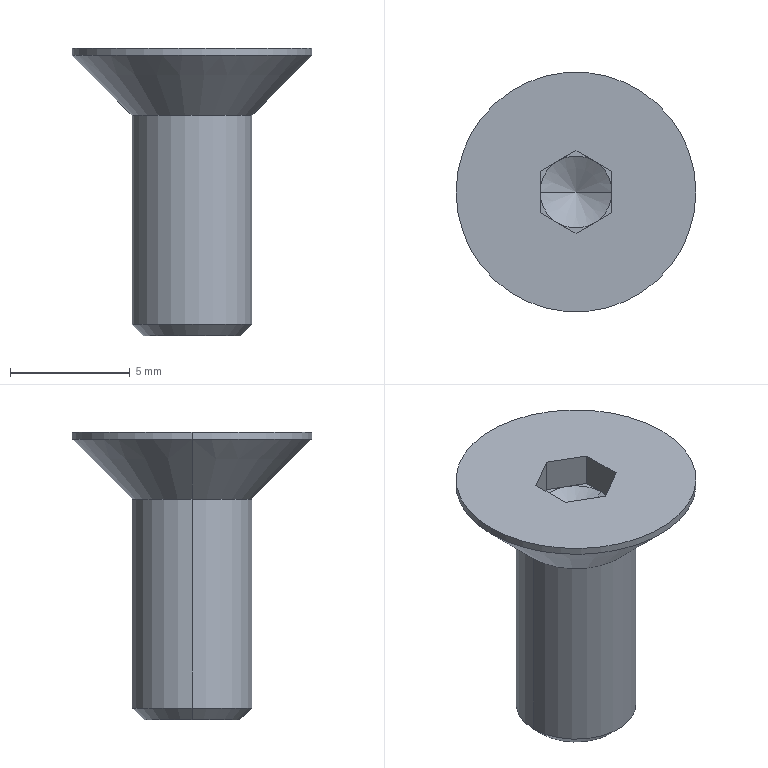Part | SolidWorks | features BaseBody 1 | 1 solid | 24 faces | box 10 x 10 x 12 mm | volume 304.022 mm3 | plane 14 | cone 6 | cylinder 4 | commonest cylinder face diameters 5 x2 10 x2
STEP:
#1=CARTESIAN_POINT('',(2.5,0.,-8.71));
#2=VERTEX_POINT('',#1);
#3=CARTESIAN_POINT('',(-2.5,0.,-8.71));
#4=VERTEX_POINT('',#3);
#5=CARTESIAN_POINT('',(0.,0.,-8.71));
#6=DIRECTION('',(0.,0.,1.));
#7=DIRECTION('',(1.,0.,0.));
#8=AXIS2_PLACEMENT_3D('',#5,#6,#7);
#9=CIRCLE('',#8,2.5);
#10=EDGE_CURVE('',#2,#4,#9,.T.);
#11=ORIENTED_EDGE('',*,*,#10,.T.);
#12=CARTESIAN_POINT('',(-2.5,0.,0.));
#13=VERTEX_POINT('',#12);
#14=CARTESIAN_POINT('',(-2.5,0.,-9.2));
#15=DIRECTION('',(0.,0.,1.));
#16=VECTOR('',#15,1000.);
#17=LINE('',#14,#16);
#18=EDGE_CURVE('',#4,#13,#17,.T.);
#19=ORIENTED_EDGE('',*,*,#18,.T.);
#20=CARTESIAN_POINT('',(2.5,0.,0.));
#21=VERTEX_POINT('',#20);
#22=CARTESIAN_POINT('',(0.,0.,0.));
#23=DIRECTION('',(0.,0.,-1.));
#24=DIRECTION('',(1.,0.,0.));
#25=AXIS2_PLACEMENT_3D('',#22,#23,#24);
#26=CIRCLE('',#25,2.5);
#27=EDGE_CURVE('',#13,#21,#26,.T.);
#28=ORIENTED_EDGE('',*,*,#27,.T.);
#29=CARTESIAN_POINT('',(2.5,0.,-9.2));
#30=DIRECTION('',(0.,0.,1.));
#31=VECTOR('',#30,1000.);
#32=LINE('',#29,#31);
#33=EDGE_CURVE('',#2,#21,#32,.T.);
#34=ORIENTED_EDGE('',*,*,#33,.F.);
#35=EDGE_LOOP('',(#11,#19,#28,#34));
#36=FACE_OUTER_BOUND('',#35,.T.);
#37=CARTESIAN_POINT('',(0.,0.,-9.2));
#38=DIRECTION('',(0.,0.,1.));
#39=DIRECTION('',(1.,0.,0.));
#40=AXIS2_PLACEMENT_3D('',#37,#38,#39);
#41=CYLINDRICAL_SURFACE('',#40,2.5);
#42=ADVANCED_FACE('',(#36),#41,.T.);
#43=ORIENTED_EDGE('',*,*,#27,.F.);
#44=CARTESIAN_POINT('',(-5.,0.,2.5));
#45=VERTEX_POINT('',#44);
#46=CARTESIAN_POINT('',(-5.,0.,2.5));
#47=DIRECTION('',(-0.7071,0.,0.7071));
#48=VECTOR('',#47,1000.);
#49=LINE('',#46,#48);
#50=EDGE_CURVE('',#13,#45,#49,.T.);
#51=ORIENTED_EDGE('',*,*,#50,.T.);
#52=CARTESIAN_POINT('',(5.,0.,2.5));
#53=VERTEX_POINT('',#52);
#54=CARTESIAN_POINT('',(0.,0.,2.5));
#55=DIRECTION('',(0.,0.,-1.));
#56=DIRECTION('',(1.,0.,0.));
#57=AXIS2_PLACEMENT_3D('',#54,#55,#56);
#58=CIRCLE('',#57,5.);
#59=EDGE_CURVE('',#45,#53,#58,.T.);
#60=ORIENTED_EDGE('',*,*,#59,.T.);
#61=CARTESIAN_POINT('',(5.,0.,2.5));
#62=DIRECTION('',(0.7071,0.,0.7071));
#63=VECTOR('',#62,1000.);
#64=LINE('',#61,#63);
#65=EDGE_CURVE('',#21,#53,#64,.T.);
#66=ORIENTED_EDGE('',*,*,#65,.F.);
#67=EDGE_LOOP('',(#43,#51,#60,#66));
#68=FACE_OUTER_BOUND('',#67,.T.);
#69=CARTESIAN_POINT('',(0.,0.,2.5));
#70=DIRECTION('',(0.,0.,1.));
#71=DIRECTION('',(1.,0.,0.));
#72=AXIS2_PLACEMENT_3D('',#69,#70,#71);
#73=CONICAL_SURFACE('',#72,5.,0.7854);
#74=ADVANCED_FACE('',(#68),#73,.T.);
#75=CARTESIAN_POINT('',(2.009,0.,-9.2));
#76=VERTEX_POINT('',#75);
#77=CARTESIAN_POINT('',(-2.009,0.,-9.2));
#78=VERTEX_POINT('',#77);
#79=CARTESIAN_POINT('',(0.,0.,-9.2));
#80=DIRECTION('',(0.,0.,1.));
#81=DIRECTION('',(1.,0.,0.));
#82=AXIS2_PLACEMENT_3D('',#79,#80,#81);
#83=CIRCLE('',#82,2.009);
#84=EDGE_CURVE('',#76,#78,#83,.T.);
#85=ORIENTED_EDGE('',*,*,#84,.T.);
#86=CARTESIAN_POINT('',(-2.5,0.,-8.71));
#87=DIRECTION('',(-0.7071,0.,0.7071));
#88=VECTOR('',#87,1000.);
#89=LINE('',#86,#88);
#90=EDGE_CURVE('',#78,#4,#89,.T.);
#91=ORIENTED_EDGE('',*,*,#90,.T.);
#92=ORIENTED_EDGE('',*,*,#10,.F.);
#93=CARTESIAN_POINT('',(2.5,0.,-8.71));
#94=DIRECTION('',(0.7071,0.,0.7071));
#95=VECTOR('',#94,1000.);
#96=LINE('',#93,#95);
#97=EDGE_CURVE('',#76,#2,#96,.T.);
#98=ORIENTED_EDGE('',*,*,#97,.F.);
#99=EDGE_LOOP('',(#85,#91,#92,#98));
#100=FACE_OUTER_BOUND('',#99,.T.);
#101=CARTESIAN_POINT('',(0.,0.,-8.71));
#102=DIRECTION('',(0.,0.,1.));
#103=DIRECTION('',(1.,0.,0.));
#104=AXIS2_PLACEMENT_3D('',#101,#102,#103);
#105=CONICAL_SURFACE('',#104,2.5,0.7854);
#106=ADVANCED_FACE('',(#100),#105,.T.);
#107=ORIENTED_EDGE('',*,*,#59,.F.);
#108=CARTESIAN_POINT('',(-5.,0.,2.8));
#109=VERTEX_POINT('',#108);
#110=CARTESIAN_POINT('',(-5.,0.,0.));
#111=DIRECTION('',(0.,0.,1.));
#112=VECTOR('',#111,1000.);
#113=LINE('',#110,#112);
#114=EDGE_CURVE('',#45,#109,#113,.T.);
#115=ORIENTED_EDGE('',*,*,#114,.T.);
#116=CARTESIAN_POINT('',(5.,0.,2.8));
#117=VERTEX_POINT('',#116);
#118=CARTESIAN_POINT('',(0.,0.,2.8));
#119=DIRECTION('',(0.,0.,-1.));
#120=DIRECTION('',(1.,0.,0.));
#121=AXIS2_PLACEMENT_3D('',#118,#119,#120);
#122=CIRCLE('',#121,5.);
#123=EDGE_CURVE('',#109,#117,#122,.T.);
#124=ORIENTED_EDGE('',*,*,#123,.T.);
#125=CARTESIAN_POINT('',(5.,0.,0.));
#126=DIRECTION('',(0.,0.,1.));
#127=VECTOR('',#126,1000.);
#128=LINE('',#125,#127);
#129=EDGE_CURVE('',#53,#117,#128,.T.);
#130=ORIENTED_EDGE('',*,*,#129,.F.);
#131=EDGE_LOOP('',(#107,#115,#124,#130));
#132=FACE_OUTER_BOUND('',#131,.T.);
#133=CARTESIAN_POINT('',(0.,0.,0.));
#134=DIRECTION('',(0.,0.,1.));
#135=DIRECTION('',(1.,0.,0.));
#136=AXIS2_PLACEMENT_3D('',#133,#134,#135);
#137=CYLINDRICAL_SURFACE('',#136,5.);
#138=ADVANCED_FACE('',(#132),#137,.T.);
#139=CARTESIAN_POINT('',(0.,0.,0.534));
#140=VERTEX_POINT('',#139);
#141=CARTESIAN_POINT('',(1.5,0.,1.4));
#142=VERTEX_POINT('',#141);
#143=CARTESIAN_POINT('',(1.5,0.,1.4));
#144=DIRECTION('',(0.866,0.,0.5));
#145=VECTOR('',#144,1000.);
#146=LINE('',#143,#145);
#147=EDGE_CURVE('',#140,#142,#146,.T.);
#148=ORIENTED_EDGE('',*,*,#147,.F.);
#149=CARTESIAN_POINT('',(-1.5,0.,1.4));
#150=VERTEX_POINT('',#149);
#151=CARTESIAN_POINT('',(-1.5,0.,1.4));
#152=DIRECTION('',(-0.866,0.,0.5));
#153=VECTOR('',#152,1000.);
#154=LINE('',#151,#153);
#155=EDGE_CURVE('',#140,#150,#154,.T.);
#156=ORIENTED_EDGE('',*,*,#155,.T.);
#157=CARTESIAN_POINT('',(-0.75,-1.299,1.4));
#158=VERTEX_POINT('',#157);
#159=CARTESIAN_POINT('',(0.,0.,1.4));
#160=DIRECTION('',(0.,0.,-1.));
#161=DIRECTION('',(1.,0.,0.));
#162=AXIS2_PLACEMENT_3D('',#159,#160,#161);
#163=CIRCLE('',#162,1.5);
#164=EDGE_CURVE('',#158,#150,#163,.T.);
#165=ORIENTED_EDGE('',*,*,#164,.F.);
#166=CARTESIAN_POINT('',(0.75,-1.299,1.4));
#167=VERTEX_POINT('',#166);
#168=CARTESIAN_POINT('',(0.,0.,1.4));
#169=DIRECTION('',(0.,0.,-1.));
#170=DIRECTION('',(1.,0.,0.));
#171=AXIS2_PLACEMENT_3D('',#168,#169,#170);
#172=CIRCLE('',#171,1.5);
#173=EDGE_CURVE('',#167,#158,#172,.T.);
#174=ORIENTED_EDGE('',*,*,#173,.F.);
#175=CARTESIAN_POINT('',(0.,0.,1.4));
#176=DIRECTION('',(0.,0.,-1.));
#177=DIRECTION('',(1.,0.,0.));
#178=AXIS2_PLACEMENT_3D('',#175,#176,#177);
#179=CIRCLE('',#178,1.5);
#180=EDGE_CURVE('',#142,#167,#179,.T.);
#181=ORIENTED_EDGE('',*,*,#180,.F.);
#182=EDGE_LOOP('',(#148,#156,#165,#174,#181));
#183=FACE_OUTER_BOUND('',#182,.T.);
#184=CARTESIAN_POINT('',(0.,0.,1.4));
#185=DIRECTION('',(0.,0.,1.));
#186=DIRECTION('',(1.,0.,0.));
#187=AXIS2_PLACEMENT_3D('',#184,#185,#186);
#188=CONICAL_SURFACE('',#187,1.5,1.047);
#189=ADVANCED_FACE('',(#183),#188,.F.);
#190=ORIENTED_EDGE('',*,*,#18,.F.);
#191=CARTESIAN_POINT('',(0.,0.,-8.71));
#192=DIRECTION('',(0.,0.,1.));
#193=DIRECTION('',(1.,0.,0.));
#194=AXIS2_PLACEMENT_3D('',#191,#192,#193);
#195=CIRCLE('',#194,2.5);
#196=EDGE_CURVE('',#4,#2,#195,.T.);
#197=ORIENTED_EDGE('',*,*,#196,.T.);
#198=ORIENTED_EDGE('',*,*,#33,.T.);
#199=CARTESIAN_POINT('',(0.,0.,0.));
#200=DIRECTION('',(0.,0.,-1.));
#201=DIRECTION('',(1.,0.,0.));
#202=AXIS2_PLACEMENT_3D('',#199,#200,#201);
#203=CIRCLE('',#202,2.5);
#204=EDGE_CURVE('',#21,#13,#203,.T.);
#205=ORIENTED_EDGE('',*,*,#204,.T.);
#206=EDGE_LOOP('',(#190,#197,#198,#205));
#207=FACE_OUTER_BOUND('',#206,.T.);
#208=CARTESIAN_POINT('',(0.,0.,-9.2));
#209=DIRECTION('',(0.,0.,1.));
#210=DIRECTION('',(1.,0.,0.));
#211=AXIS2_PLACEMENT_3D('',#208,#209,#210);
#212=CYLINDRICAL_SURFACE('',#211,2.5);
#213=ADVANCED_FACE('',(#207),#212,.T.);
#214=ORIENTED_EDGE('',*,*,#50,.F.);
#215=ORIENTED_EDGE('',*,*,#204,.F.);
#216=ORIENTED_EDGE('',*,*,#65,.T.);
#217=CARTESIAN_POINT('',(0.,0.,2.5));
#218=DIRECTION('',(0.,0.,-1.));
#219=DIRECTION('',(1.,0.,0.));
#220=AXIS2_PLACEMENT_3D('',#217,#218,#219);
#221=CIRCLE('',#220,5.);
#222=EDGE_CURVE('',#53,#45,#221,.T.);
#223=ORIENTED_EDGE('',*,*,#222,.T.);
#224=EDGE_LOOP('',(#214,#215,#216,#223));
#225=FACE_OUTER_BOUND('',#224,.T.);
#226=CARTESIAN_POINT('',(0.,0.,2.5));
#227=DIRECTION('',(0.,0.,1.));
#228=DIRECTION('',(1.,0.,0.));
#229=AXIS2_PLACEMENT_3D('',#226,#227,#228);
#230=CONICAL_SURFACE('',#229,5.,0.7854);
#231=ADVANCED_FACE('',(#225),#230,.T.);
#232=ORIENTED_EDGE('',*,*,#90,.F.);
#233=CARTESIAN_POINT('',(0.,0.,-9.2));
#234=DIRECTION('',(0.,0.,1.));
#235=DIRECTION('',(1.,0.,0.));
#236=AXIS2_PLACEMENT_3D('',#233,#234,#235);
#237=CIRCLE('',#236,2.009);
#238=EDGE_CURVE('',#78,#76,#237,.T.);
#239=ORIENTED_EDGE('',*,*,#238,.T.);
#240=ORIENTED_EDGE('',*,*,#97,.T.);
#241=ORIENTED_EDGE('',*,*,#196,.F.);
#242=EDGE_LOOP('',(#232,#239,#240,#241));
#243=FACE_OUTER_BOUND('',#242,.T.);
#244=CARTESIAN_POINT('',(0.,0.,-8.71));
#245=DIRECTION('',(0.,0.,1.));
#246=DIRECTION('',(1.,0.,0.));
#247=AXIS2_PLACEMENT_3D('',#244,#245,#246);
#248=CONICAL_SURFACE('',#247,2.5,0.7854);
#249=ADVANCED_FACE('',(#243),#248,.T.);
#250=ORIENTED_EDGE('',*,*,#114,.F.);
#251=ORIENTED_EDGE('',*,*,#222,.F.);
#252=ORIENTED_EDGE('',*,*,#129,.T.);
#253=CARTESIAN_POINT('',(0.,0.,2.8));
#254=DIRECTION('',(0.,0.,-1.));
#255=DIRECTION('',(1.,0.,0.));
#256=AXIS2_PLACEMENT_3D('',#253,#254,#255);
#257=CIRCLE('',#256,5.);
#258=EDGE_CURVE('',#117,#109,#257,.T.);
#259=ORIENTED_EDGE('',*,*,#258,.T.);
#260=EDGE_LOOP('',(#250,#251,#252,#259));
#261=FACE_OUTER_BOUND('',#260,.T.);
#262=CARTESIAN_POINT('',(0.,0.,0.));
#263=DIRECTION('',(0.,0.,1.));
#264=DIRECTION('',(1.,0.,0.));
#265=AXIS2_PLACEMENT_3D('',#262,#263,#264);
#266=CYLINDRICAL_SURFACE('',#265,5.);
#267=ADVANCED_FACE('',(#261),#266,.T.);
#268=ORIENTED_EDGE('',*,*,#84,.F.);
#269=ORIENTED_EDGE('',*,*,#238,.F.);
#270=EDGE_LOOP('',(#268,#269));
#271=FACE_OUTER_BOUND('',#270,.T.);
#272=CARTESIAN_POINT('',(0.,2.01,-9.2));
#273=DIRECTION('',(0.,0.,1.));
#274=DIRECTION('',(1.,0.,0.));
#275=AXIS2_PLACEMENT_3D('',#272,#273,#274);
#276=PLANE('',#275);
#277=ADVANCED_FACE('',(#271),#276,.F.);
#278=CARTESIAN_POINT('',(-1.5,-0.866,2.8));
#279=VERTEX_POINT('',#278);
#280=CARTESIAN_POINT('',(0.,-1.732,2.8));
#281=VERTEX_POINT('',#280);
#282=CARTESIAN_POINT('',(-1.5,-0.866,2.8));
#283=DIRECTION('',(0.866,-0.5,0.));
#284=VECTOR('',#283,1000.);
#285=LINE('',#282,#284);
#286=EDGE_CURVE('',#279,#281,#285,.T.);
#287=ORIENTED_EDGE('',*,*,#286,.F.);
#288=CARTESIAN_POINT('',(-1.5,0.866,2.8));
#289=VERTEX_POINT('',#288);
#290=CARTESIAN_POINT('',(-1.5,0.,2.8));
#291=DIRECTION('',(0.,-1.,0.));
#292=VECTOR('',#291,1000.);
#293=LINE('',#290,#292);
#294=EDGE_CURVE('',#289,#279,#293,.T.);
#295=ORIENTED_EDGE('',*,*,#294,.F.);
#296=CARTESIAN_POINT('',(0.,1.732,2.8));
#297=VERTEX_POINT('',#296);
#298=CARTESIAN_POINT('',(0.,1.732,2.8));
#299=DIRECTION('',(-0.866,-0.5,0.));
#300=VECTOR('',#299,1000.);
#301=LINE('',#298,#300);
#302=EDGE_CURVE('',#297,#289,#301,.T.);
#303=ORIENTED_EDGE('',*,*,#302,.F.);
#304=CARTESIAN_POINT('',(1.5,0.866,2.8));
#305=VERTEX_POINT('',#304);
#306=CARTESIAN_POINT('',(1.5,0.866,2.8));
#307=DIRECTION('',(-0.866,0.5,0.));
#308=VECTOR('',#307,1000.);
#309=LINE('',#306,#308);
#310=EDGE_CURVE('',#305,#297,#309,.T.);
#311=ORIENTED_EDGE('',*,*,#310,.F.);
#312=CARTESIAN_POINT('',(1.5,-0.866,2.8));
#313=VERTEX_POINT('',#312);
#314=CARTESIAN_POINT('',(1.5,0.,2.8));
#315=DIRECTION('',(0.,1.,0.));
#316=VECTOR('',#315,1000.);
#317=LINE('',#314,#316);
#318=EDGE_CURVE('',#313,#305,#317,.T.);
#319=ORIENTED_EDGE('',*,*,#318,.F.);
#320=CARTESIAN_POINT('',(0.,-1.732,2.8));
#321=DIRECTION('',(0.866,0.5,0.));
#322=VECTOR('',#321,1000.);
#323=LINE('',#320,#322);
#324=EDGE_CURVE('',#281,#313,#323,.T.);
#325=ORIENTED_EDGE('',*,*,#324,.F.);
#326=EDGE_LOOP('',(#287,#295,#303,#311,#319,#325));
#327=FACE_BOUND('',#326,.T.);
#328=ORIENTED_EDGE('',*,*,#258,.F.);
#329=ORIENTED_EDGE('',*,*,#123,.F.);
#330=EDGE_LOOP('',(#328,#329));
#331=FACE_OUTER_BOUND('',#330,.T.);
#332=CARTESIAN_POINT('',(0.,0.,2.8));
#333=DIRECTION('',(0.,0.,-1.));
#334=DIRECTION('',(-1.,0.,0.));
#335=AXIS2_PLACEMENT_3D('',#332,#333,#334);
#336=PLANE('',#335);
#337=ADVANCED_FACE('',(#327,#331),#336,.F.);
#338=CARTESIAN_POINT('',(1.5,-0.866,1.4));
#339=VERTEX_POINT('',#338);
#340=CARTESIAN_POINT('',(1.5,-0.866,1.4));
#341=DIRECTION('',(0.,0.,1.));
#342=VECTOR('',#341,1000.);
#343=LINE('',#340,#342);
#344=EDGE_CURVE('',#339,#313,#343,.T.);
#345=ORIENTED_EDGE('',*,*,#344,.F.);
#346=CARTESIAN_POINT('',(0.,-1.732,1.4));
#347=DIRECTION('',(0.866,0.5,0.));
#348=VECTOR('',#347,1000.);
#349=LINE('',#346,#348);
#350=EDGE_CURVE('',#167,#339,#349,.T.);
#351=ORIENTED_EDGE('',*,*,#350,.F.);
#352=CARTESIAN_POINT('',(0.,-1.732,1.4));
#353=VERTEX_POINT('',#352);
#354=CARTESIAN_POINT('',(0.,-1.732,1.4));
#355=DIRECTION('',(0.866,0.5,0.));
#356=VECTOR('',#355,1000.);
#357=LINE('',#354,#356);
#358=EDGE_CURVE('',#353,#167,#357,.T.);
#359=ORIENTED_EDGE('',*,*,#358,.F.);
#360=CARTESIAN_POINT('',(0.,-1.732,1.4));
#361=DIRECTION('',(0.,0.,-1.));
#362=VECTOR('',#361,1000.);
#363=LINE('',#360,#362);
#364=EDGE_CURVE('',#281,#353,#363,.T.);
#365=ORIENTED_EDGE('',*,*,#364,.F.);
#366=ORIENTED_EDGE('',*,*,#324,.T.);
#367=EDGE_LOOP('',(#345,#351,#359,#365,#366));
#368=FACE_OUTER_BOUND('',#367,.T.);
#369=CARTESIAN_POINT('',(0.,-1.732,1.4));
#370=DIRECTION('',(0.5,-0.866,0.));
#371=DIRECTION('',(0.866,0.5,0.));
#372=AXIS2_PLACEMENT_3D('',#369,#370,#371);
#373=PLANE('',#372);
#374=ADVANCED_FACE('',(#368),#373,.F.);
#375=ORIENTED_EDGE('',*,*,#364,.T.);
#376=CARTESIAN_POINT('',(-1.5,-0.866,1.4));
#377=DIRECTION('',(0.866,-0.5,0.));
#378=VECTOR('',#377,1000.);
#379=LINE('',#376,#378);
#380=EDGE_CURVE('',#158,#353,#379,.T.);
#381=ORIENTED_EDGE('',*,*,#380,.F.);
#382=CARTESIAN_POINT('',(-1.5,-0.866,1.4));
#383=VERTEX_POINT('',#382);
#384=CARTESIAN_POINT('',(-1.5,-0.866,1.4));
#385=DIRECTION('',(0.866,-0.5,0.));
#386=VECTOR('',#385,1000.);
#387=LINE('',#384,#386);
#388=EDGE_CURVE('',#383,#158,#387,.T.);
#389=ORIENTED_EDGE('',*,*,#388,.F.);
#390=CARTESIAN_POINT('',(-1.5,-0.866,1.4));
#391=DIRECTION('',(0.,0.,-1.));
#392=VECTOR('',#391,1000.);
#393=LINE('',#390,#392);
#394=EDGE_CURVE('',#279,#383,#393,.T.);
#395=ORIENTED_EDGE('',*,*,#394,.F.);
#396=ORIENTED_EDGE('',*,*,#286,.T.);
#397=EDGE_LOOP('',(#375,#381,#389,#395,#396));
#398=FACE_OUTER_BOUND('',#397,.T.);
#399=CARTESIAN_POINT('',(-1.5,-0.866,1.4));
#400=DIRECTION('',(-0.5,-0.866,0.));
#401=DIRECTION('',(0.866,-0.5,0.));
#402=AXIS2_PLACEMENT_3D('',#399,#400,#401);
#403=PLANE('',#402);
#404=ADVANCED_FACE('',(#398),#403,.F.);
#405=ORIENTED_EDGE('',*,*,#394,.T.);
#406=CARTESIAN_POINT('',(-1.5,0.866,1.4));
#407=DIRECTION('',(0.,-1.,0.));
#408=VECTOR('',#407,1000.);
#409=LINE('',#406,#408);
#410=EDGE_CURVE('',#150,#383,#409,.T.);
#411=ORIENTED_EDGE('',*,*,#410,.F.);
#412=CARTESIAN_POINT('',(-1.5,0.866,1.4));
#413=VERTEX_POINT('',#412);
#414=CARTESIAN_POINT('',(-1.5,0.866,1.4));
#415=DIRECTION('',(0.,-1.,0.));
#416=VECTOR('',#415,1000.);
#417=LINE('',#414,#416);
#418=EDGE_CURVE('',#413,#150,#417,.T.);
#419=ORIENTED_EDGE('',*,*,#418,.F.);
#420=CARTESIAN_POINT('',(-1.5,0.866,1.4));
#421=DIRECTION('',(0.,0.,-1.));
#422=VECTOR('',#421,1000.);
#423=LINE('',#420,#422);
#424=EDGE_CURVE('',#289,#413,#423,.T.);
#425=ORIENTED_EDGE('',*,*,#424,.F.);
#426=ORIENTED_EDGE('',*,*,#294,.T.);
#427=EDGE_LOOP('',(#405,#411,#419,#425,#426));
#428=FACE_OUTER_BOUND('',#427,.T.);
#429=CARTESIAN_POINT('',(-1.5,0.866,1.4));
#430=DIRECTION('',(-1.,0.,0.));
#431=DIRECTION('',(0.,0.,1.));
#432=AXIS2_PLACEMENT_3D('',#429,#430,#431);
#433=PLANE('',#432);
#434=ADVANCED_FACE('',(#428),#433,.F.);
#435=ORIENTED_EDGE('',*,*,#424,.T.);
#436=CARTESIAN_POINT('',(-0.75,1.299,1.4));
#437=VERTEX_POINT('',#436);
#438=CARTESIAN_POINT('',(0.,1.732,1.4));
#439=DIRECTION('',(-0.866,-0.5,0.));
#440=VECTOR('',#439,1000.);
#441=LINE('',#438,#440);
#442=EDGE_CURVE('',#437,#413,#441,.T.);
#443=ORIENTED_EDGE('',*,*,#442,.F.);
#444=CARTESIAN_POINT('',(0.,1.732,1.4));
#445=VERTEX_POINT('',#444);
#446=CARTESIAN_POINT('',(0.,1.732,1.4));
#447=DIRECTION('',(-0.866,-0.5,0.));
#448=VECTOR('',#447,1000.);
#449=LINE('',#446,#448);
#450=EDGE_CURVE('',#445,#437,#449,.T.);
#451=ORIENTED_EDGE('',*,*,#450,.F.);
#452=CARTESIAN_POINT('',(0.,1.732,1.4));
#453=DIRECTION('',(0.,0.,-1.));
#454=VECTOR('',#453,1000.);
#455=LINE('',#452,#454);
#456=EDGE_CURVE('',#297,#445,#455,.T.);
#457=ORIENTED_EDGE('',*,*,#456,.F.);
#458=ORIENTED_EDGE('',*,*,#302,.T.);
#459=EDGE_LOOP('',(#435,#443,#451,#457,#458));
#460=FACE_OUTER_BOUND('',#459,.T.);
#461=CARTESIAN_POINT('',(0.,1.732,1.4));
#462=DIRECTION('',(-0.5,0.866,0.));
#463=DIRECTION('',(-0.866,-0.5,0.));
#464=AXIS2_PLACEMENT_3D('',#461,#462,#463);
#465=PLANE('',#464);
#466=ADVANCED_FACE('',(#460),#465,.F.);
#467=ORIENTED_EDGE('',*,*,#456,.T.);
#468=CARTESIAN_POINT('',(0.75,1.299,1.4));
#469=VERTEX_POINT('',#468);
#470=CARTESIAN_POINT('',(1.5,0.866,1.4));
#471=DIRECTION('',(-0.866,0.5,0.));
#472=VECTOR('',#471,1000.);
#473=LINE('',#470,#472);
#474=EDGE_CURVE('',#469,#445,#473,.T.);
#475=ORIENTED_EDGE('',*,*,#474,.F.);
#476=CARTESIAN_POINT('',(1.5,0.866,1.4));
#477=VERTEX_POINT('',#476);
#478=CARTESIAN_POINT('',(1.5,0.866,1.4));
#479=DIRECTION('',(-0.866,0.5,0.));
#480=VECTOR('',#479,1000.);
#481=LINE('',#478,#480);
#482=EDGE_CURVE('',#477,#469,#481,.T.);
#483=ORIENTED_EDGE('',*,*,#482,.F.);
#484=CARTESIAN_POINT('',(1.5,0.866,1.4));
#485=DIRECTION('',(0.,0.,-1.));
#486=VECTOR('',#485,1000.);
#487=LINE('',#484,#486);
#488=EDGE_CURVE('',#305,#477,#487,.T.);
#489=ORIENTED_EDGE('',*,*,#488,.F.);
#490=ORIENTED_EDGE('',*,*,#310,.T.);
#491=EDGE_LOOP('',(#467,#475,#483,#489,#490));
#492=FACE_OUTER_BOUND('',#491,.T.);
#493=CARTESIAN_POINT('',(1.5,0.866,1.4));
#494=DIRECTION('',(0.5,0.866,0.));
#495=DIRECTION('',(-0.866,0.5,0.));
#496=AXIS2_PLACEMENT_3D('',#493,#494,#495);
#497=PLANE('',#496);
#498=ADVANCED_FACE('',(#492),#497,.F.);
#499=ORIENTED_EDGE('',*,*,#488,.T.);
#500=CARTESIAN_POINT('',(1.5,-0.866,1.4));
#501=DIRECTION('',(0.,1.,0.));
#502=VECTOR('',#501,1000.);
#503=LINE('',#500,#502);
#504=EDGE_CURVE('',#142,#477,#503,.T.);
#505=ORIENTED_EDGE('',*,*,#504,.F.);
#506=CARTESIAN_POINT('',(1.5,-0.866,1.4));
#507=DIRECTION('',(0.,1.,0.));
#508=VECTOR('',#507,1000.);
#509=LINE('',#506,#508);
#510=EDGE_CURVE('',#339,#142,#509,.T.);
#511=ORIENTED_EDGE('',*,*,#510,.F.);
#512=ORIENTED_EDGE('',*,*,#344,.T.);
#513=ORIENTED_EDGE('',*,*,#318,.T.);
#514=EDGE_LOOP('',(#499,#505,#511,#512,#513));
#515=FACE_OUTER_BOUND('',#514,.T.);
#516=CARTESIAN_POINT('',(1.5,-0.866,1.4));
#517=DIRECTION('',(1.,0.,0.));
#518=DIRECTION('',(0.,0.,-1.));
#519=AXIS2_PLACEMENT_3D('',#516,#517,#518);
#520=PLANE('',#519);
#521=ADVANCED_FACE('',(#515),#520,.F.);
#522=ORIENTED_EDGE('',*,*,#180,.T.);
#523=ORIENTED_EDGE('',*,*,#350,.T.);
#524=ORIENTED_EDGE('',*,*,#510,.T.);
#525=EDGE_LOOP('',(#522,#523,#524));
#526=FACE_OUTER_BOUND('',#525,.T.);
#527=CARTESIAN_POINT('',(0.,0.,1.4));
#528=DIRECTION('',(0.,0.,1.));
#529=DIRECTION('',(1.,0.,0.));
#530=AXIS2_PLACEMENT_3D('',#527,#528,#529);
#531=PLANE('',#530);
#532=ADVANCED_FACE('',(#526),#531,.T.);
#533=ORIENTED_EDGE('',*,*,#173,.T.);
#534=ORIENTED_EDGE('',*,*,#380,.T.);
#535=ORIENTED_EDGE('',*,*,#358,.T.);
#536=EDGE_LOOP('',(#533,#534,#535));
#537=FACE_OUTER_BOUND('',#536,.T.);
#538=CARTESIAN_POINT('',(0.,0.,1.4));
#539=DIRECTION('',(0.,0.,1.));
#540=DIRECTION('',(1.,0.,0.));
#541=AXIS2_PLACEMENT_3D('',#538,#539,#540);
#542=PLANE('',#541);
#543=ADVANCED_FACE('',(#537),#542,.T.);
#544=ORIENTED_EDGE('',*,*,#164,.T.);
#545=ORIENTED_EDGE('',*,*,#410,.T.);
#546=ORIENTED_EDGE('',*,*,#388,.T.);
#547=EDGE_LOOP('',(#544,#545,#546));
#548=FACE_OUTER_BOUND('',#547,.T.);
#549=CARTESIAN_POINT('',(0.,0.,1.4));
#550=DIRECTION('',(0.,0.,1.));
#551=DIRECTION('',(1.,0.,0.));
#552=AXIS2_PLACEMENT_3D('',#549,#550,#551);
#553=PLANE('',#552);
#554=ADVANCED_FACE('',(#548),#553,.T.);
#555=CARTESIAN_POINT('',(0.,0.,1.4));
#556=DIRECTION('',(0.,0.,-1.));
#557=DIRECTION('',(1.,0.,0.));
#558=AXIS2_PLACEMENT_3D('',#555,#556,#557);
#559=CIRCLE('',#558,1.5);
#560=EDGE_CURVE('',#150,#437,#559,.T.);
#561=ORIENTED_EDGE('',*,*,#560,.T.);
#562=ORIENTED_EDGE('',*,*,#442,.T.);
#563=ORIENTED_EDGE('',*,*,#418,.T.);
#564=EDGE_LOOP('',(#561,#562,#563));
#565=FACE_OUTER_BOUND('',#564,.T.);
#566=CARTESIAN_POINT('',(0.,0.,1.4));
#567=DIRECTION('',(0.,0.,1.));
#568=DIRECTION('',(1.,0.,0.));
#569=AXIS2_PLACEMENT_3D('',#566,#567,#568);
#570=PLANE('',#569);
#571=ADVANCED_FACE('',(#565),#570,.T.);
#572=CARTESIAN_POINT('',(0.,0.,1.4));
#573=DIRECTION('',(0.,0.,-1.));
#574=DIRECTION('',(1.,0.,0.));
#575=AXIS2_PLACEMENT_3D('',#572,#573,#574);
#576=CIRCLE('',#575,1.5);
#577=EDGE_CURVE('',#437,#469,#576,.T.);
#578=ORIENTED_EDGE('',*,*,#577,.T.);
#579=ORIENTED_EDGE('',*,*,#474,.T.);
#580=ORIENTED_EDGE('',*,*,#450,.T.);
#581=EDGE_LOOP('',(#578,#579,#580));
#582=FACE_OUTER_BOUND('',#581,.T.);
#583=CARTESIAN_POINT('',(0.,0.,1.4));
#584=DIRECTION('',(0.,0.,1.));
#585=DIRECTION('',(1.,0.,0.));
#586=AXIS2_PLACEMENT_3D('',#583,#584,#585);
#587=PLANE('',#586);
#588=ADVANCED_FACE('',(#582),#587,.T.);
#589=CARTESIAN_POINT('',(0.,0.,1.4));
#590=DIRECTION('',(0.,0.,-1.));
#591=DIRECTION('',(1.,0.,0.));
#592=AXIS2_PLACEMENT_3D('',#589,#590,#591);
#593=CIRCLE('',#592,1.5);
#594=EDGE_CURVE('',#469,#142,#593,.T.);
#595=ORIENTED_EDGE('',*,*,#594,.T.);
#596=ORIENTED_EDGE('',*,*,#504,.T.);
#597=ORIENTED_EDGE('',*,*,#482,.T.);
#598=EDGE_LOOP('',(#595,#596,#597));
#599=FACE_OUTER_BOUND('',#598,.T.);
#600=CARTESIAN_POINT('',(0.,0.,1.4));
#601=DIRECTION('',(0.,0.,1.));
#602=DIRECTION('',(1.,0.,0.));
#603=AXIS2_PLACEMENT_3D('',#600,#601,#602);
#604=PLANE('',#603);
#605=ADVANCED_FACE('',(#599),#604,.T.);
#606=ORIENTED_EDGE('',*,*,#155,.F.);
#607=ORIENTED_EDGE('',*,*,#147,.T.);
#608=ORIENTED_EDGE('',*,*,#594,.F.);
#609=ORIENTED_EDGE('',*,*,#577,.F.);
#610=ORIENTED_EDGE('',*,*,#560,.F.);
#611=EDGE_LOOP('',(#606,#607,#608,#609,#610));
#612=FACE_OUTER_BOUND('',#611,.T.);
#613=CARTESIAN_POINT('',(0.,0.,1.4));
#614=DIRECTION('',(0.,0.,1.));
#615=DIRECTION('',(1.,0.,0.));
#616=AXIS2_PLACEMENT_3D('',#613,#614,#615);
#617=CONICAL_SURFACE('',#616,1.5,1.047);
#618=ADVANCED_FACE('',(#612),#617,.F.);
#619=CLOSED_SHELL('',(#42,#74,#106,#138,#189,#213,#231,#249,#267,#277,#337,#374,#404,#434,#466,#498,#521,#532,#543,#554,#571,#588,#605,#618));
#620=MANIFOLD_SOLID_BREP('',#619);
#621=CARTESIAN_POINT('',(0.,0.,0.));
#622=DIRECTION('',(0.,0.,1.));
#623=DIRECTION('',(1.,0.,0.));
#624=AXIS2_PLACEMENT_3D('',#621,#622,#623);
#625=(LENGTH_UNIT()NAMED_UNIT(*)SI_UNIT(.MILLI.,.METRE.));
#626=UNCERTAINTY_MEASURE_WITH_UNIT(LENGTH_MEASURE(0.00001),#625,'','');
#627=(NAMED_UNIT(*)PLANE_ANGLE_UNIT()SI_UNIT($,.RADIAN.));
#628=(NAMED_UNIT(*)SI_UNIT($,.STERADIAN.)SOLID_ANGLE_UNIT());
#629=(GEOMETRIC_REPRESENTATION_CONTEXT(3)GLOBAL_UNCERTAINTY_ASSIGNED_CONTEXT((#626))GLOBAL_UNIT_ASSIGNED_CONTEXT((#625,#627,#628))REPRESENTATION_CONTEXT('',''));
#630=ADVANCED_BREP_SHAPE_REPRESENTATION('',(#620,#624),#629);